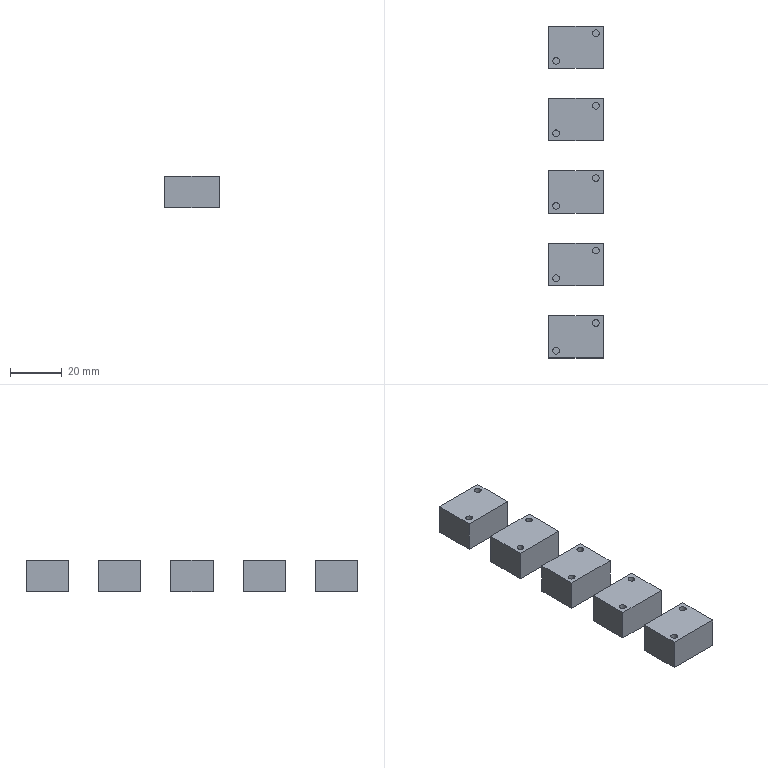NC program | NX | posted with a generic post | part box 21 x 128.262 x 12 mm
Whole program:
N10 G17 G21 G94 G90
(PLANAR_MILL_COPY , TOOL : D6A45)
N12 T07 M6
N14 G54
N16 G17 G0 G90 X65.388 Y0.766 S9500 M3
N18 G43 Z30. H7
N20 Z0.5
N22 G94 G1 Z-1. F1250.
N24 G3 X65.031 Y0. R1.
N26 G1 Y-10.5
N28 G2 X64.131 Y-11.4 R0.9
N30 G1 X47.869
N32 G2 X46.969 Y-10.5 R0.9
N34 G1 Y10.5
N36 G2 X47.869 Y11.4 R0.9
N38 G1 X64.131
N40 G2 X65.031 Y10.5 R0.9
N42 G1 Y0.
N44 G3 X65.388 Y-0.766 R1.
N46 G1 Z0.5
N48 G0 Z30.
N50 X37.388 Y0.766
N52 Z0.5
N54 G1 Z-1.
N56 G3 X37.031 Y0. R1.
N58 G1 Y-10.5
N60 G2 X36.131 Y-11.4 R0.9
N62 G1 X19.869
N64 G2 X18.969 Y-10.5 R0.9
N66 G1 Y10.5
N68 G2 X19.869 Y11.4 R0.9
N70 G1 X36.131
N72 G2 X37.031 Y10.5 R0.9
N74 G1 Y0.
N76 G3 X37.388 Y-0.766 R1.
N78 G1 Z0.5
N80 G0 Z30.
N82 X9.388 Y0.766
N84 Z0.5
N86 G1 Z-1.
N88 G3 X9.031 Y0. R1.
N90 G1 Y-10.5
N92 G2 X8.131 Y-11.4 R0.9
N94 G1 X-8.131
N96 G2 X-9.031 Y-10.5 R0.9
N98 G1 Y10.5
N100 G2 X-8.131 Y11.4 R0.9
N102 G1 X8.131
N104 G2 X9.031 Y10.5 R0.9
N106 G1 Y0.
N108 G3 X9.388 Y-0.766 R1.
N110 G1 Z0.5
N112 G0 Z30.
N114 X-18.612 Y0.766
N116 Z0.5
N118 G1 Z-1.
N120 G3 X-18.969 Y0. R1.
N122 G1 Y-10.5
N124 G2 X-19.869 Y-11.4 R0.9
N126 G1 X-36.131
N128 G2 X-37.031 Y-10.5 R0.9
N130 G1 Y10.5
N132 G2 X-36.131 Y11.4 R0.9
N134 G1 X-19.869
N136 G2 X-18.969 Y10.5 R0.9
N138 G1 Y0.
N140 G3 X-18.612 Y-0.766 R1.
N142 G1 Z0.5
N144 G0 Z30.
N146 X-46.612 Y0.766
N148 Z0.5
N150 G1 Z-1.
N152 G3 X-46.969 Y0. R1.
N154 G1 Y-10.5
N156 G2 X-47.869 Y-11.4 R0.9
N158 G1 X-64.131
N160 G2 X-65.031 Y-10.5 R0.9
N162 G1 Y10.5
N164 G2 X-64.131 Y11.4 R0.9
N166 G1 X-47.869
N168 G2 X-46.969 Y10.5 R0.9
N170 G1 Y0.
N172 G3 X-46.612 Y-0.766 R1.
N174 G1 Z0.5
N176 G0 Z30.
N178 M5
N180 M2